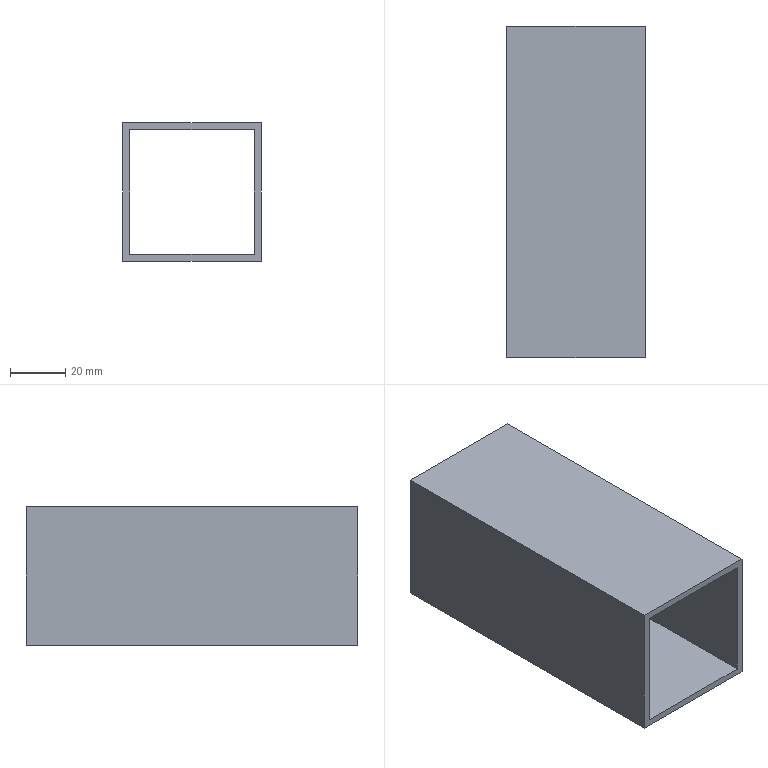Part | STEP file | MB-P-20 | 1 solid | 10 faces | box 50 x 120 x 50 mm | volume 57000 mm3 | plane 10
STEP:
#1=CARTESIAN_POINT('',(2.5,120.,4.5));
#2=VERTEX_POINT('',#1);
#3=CARTESIAN_POINT('',(47.5,120.,4.5));
#4=VERTEX_POINT('',#3);
#5=CARTESIAN_POINT('',(2.5,120.,4.5));
#6=DIRECTION('',(1.,0.,0.));
#7=VECTOR('',#6,1000.);
#8=LINE('',#5,#7);
#9=EDGE_CURVE('',#2,#4,#8,.T.);
#10=ORIENTED_EDGE('',*,*,#9,.T.);
#11=CARTESIAN_POINT('',(47.5,120.,49.5));
#12=VERTEX_POINT('',#11);
#13=CARTESIAN_POINT('',(47.5,120.,4.5));
#14=DIRECTION('',(0.,0.,1.));
#15=VECTOR('',#14,1000.);
#16=LINE('',#13,#15);
#17=EDGE_CURVE('',#4,#12,#16,.T.);
#18=ORIENTED_EDGE('',*,*,#17,.T.);
#19=CARTESIAN_POINT('',(2.5,120.,49.5));
#20=VERTEX_POINT('',#19);
#21=CARTESIAN_POINT('',(47.5,120.,49.5));
#22=DIRECTION('',(-1.,0.,0.));
#23=VECTOR('',#22,1000.);
#24=LINE('',#21,#23);
#25=EDGE_CURVE('',#12,#20,#24,.T.);
#26=ORIENTED_EDGE('',*,*,#25,.T.);
#27=CARTESIAN_POINT('',(2.5,120.,49.5));
#28=DIRECTION('',(0.,0.,-1.));
#29=VECTOR('',#28,1000.);
#30=LINE('',#27,#29);
#31=EDGE_CURVE('',#20,#2,#30,.T.);
#32=ORIENTED_EDGE('',*,*,#31,.T.);
#33=EDGE_LOOP('',(#10,#18,#26,#32));
#34=FACE_BOUND('',#33,.T.);
#35=CARTESIAN_POINT('',(0.,120.,2.));
#36=VERTEX_POINT('',#35);
#37=CARTESIAN_POINT('',(0.,120.,52.));
#38=VERTEX_POINT('',#37);
#39=CARTESIAN_POINT('',(0.,120.,52.));
#40=DIRECTION('',(0.,0.,1.));
#41=VECTOR('',#40,1000.);
#42=LINE('',#39,#41);
#43=EDGE_CURVE('',#36,#38,#42,.T.);
#44=ORIENTED_EDGE('',*,*,#43,.T.);
#45=CARTESIAN_POINT('',(50.,120.,52.));
#46=VERTEX_POINT('',#45);
#47=CARTESIAN_POINT('',(50.,120.,52.));
#48=DIRECTION('',(1.,0.,0.));
#49=VECTOR('',#48,1000.);
#50=LINE('',#47,#49);
#51=EDGE_CURVE('',#38,#46,#50,.T.);
#52=ORIENTED_EDGE('',*,*,#51,.T.);
#53=CARTESIAN_POINT('',(50.,120.,2.));
#54=VERTEX_POINT('',#53);
#55=CARTESIAN_POINT('',(50.,120.,2.));
#56=DIRECTION('',(0.,0.,-1.));
#57=VECTOR('',#56,1000.);
#58=LINE('',#55,#57);
#59=EDGE_CURVE('',#46,#54,#58,.T.);
#60=ORIENTED_EDGE('',*,*,#59,.T.);
#61=CARTESIAN_POINT('',(0.,120.,2.));
#62=DIRECTION('',(-1.,0.,0.));
#63=VECTOR('',#62,1000.);
#64=LINE('',#61,#63);
#65=EDGE_CURVE('',#54,#36,#64,.T.);
#66=ORIENTED_EDGE('',*,*,#65,.T.);
#67=EDGE_LOOP('',(#44,#52,#60,#66));
#68=FACE_OUTER_BOUND('',#67,.T.);
#69=CARTESIAN_POINT('',(25.,120.,27.));
#70=DIRECTION('',(0.,1.,0.));
#71=DIRECTION('',(1.,0.,0.));
#72=AXIS2_PLACEMENT_3D('',#69,#70,#71);
#73=PLANE('',#72);
#74=ADVANCED_FACE('',(#34,#68),#73,.T.);
#75=CARTESIAN_POINT('',(47.5,0.,4.5));
#76=VERTEX_POINT('',#75);
#77=CARTESIAN_POINT('',(2.5,0.,4.5));
#78=VERTEX_POINT('',#77);
#79=CARTESIAN_POINT('',(2.5,0.,4.5));
#80=DIRECTION('',(-1.,0.,0.));
#81=VECTOR('',#80,1000.);
#82=LINE('',#79,#81);
#83=EDGE_CURVE('',#76,#78,#82,.T.);
#84=ORIENTED_EDGE('',*,*,#83,.T.);
#85=CARTESIAN_POINT('',(2.5,0.,49.5));
#86=VERTEX_POINT('',#85);
#87=CARTESIAN_POINT('',(2.5,0.,49.5));
#88=DIRECTION('',(0.,0.,1.));
#89=VECTOR('',#88,1000.);
#90=LINE('',#87,#89);
#91=EDGE_CURVE('',#78,#86,#90,.T.);
#92=ORIENTED_EDGE('',*,*,#91,.T.);
#93=CARTESIAN_POINT('',(47.5,0.,49.5));
#94=VERTEX_POINT('',#93);
#95=CARTESIAN_POINT('',(47.5,0.,49.5));
#96=DIRECTION('',(1.,0.,0.));
#97=VECTOR('',#96,1000.);
#98=LINE('',#95,#97);
#99=EDGE_CURVE('',#86,#94,#98,.T.);
#100=ORIENTED_EDGE('',*,*,#99,.T.);
#101=CARTESIAN_POINT('',(47.5,0.,4.5));
#102=DIRECTION('',(0.,0.,-1.));
#103=VECTOR('',#102,1000.);
#104=LINE('',#101,#103);
#105=EDGE_CURVE('',#94,#76,#104,.T.);
#106=ORIENTED_EDGE('',*,*,#105,.T.);
#107=EDGE_LOOP('',(#84,#92,#100,#106));
#108=FACE_BOUND('',#107,.T.);
#109=CARTESIAN_POINT('',(0.,0.,52.));
#110=VERTEX_POINT('',#109);
#111=CARTESIAN_POINT('',(0.,0.,2.));
#112=VERTEX_POINT('',#111);
#113=CARTESIAN_POINT('',(0.,0.,52.));
#114=DIRECTION('',(0.,0.,-1.));
#115=VECTOR('',#114,1000.);
#116=LINE('',#113,#115);
#117=EDGE_CURVE('',#110,#112,#116,.T.);
#118=ORIENTED_EDGE('',*,*,#117,.T.);
#119=CARTESIAN_POINT('',(50.,0.,2.));
#120=VERTEX_POINT('',#119);
#121=CARTESIAN_POINT('',(0.,0.,2.));
#122=DIRECTION('',(1.,0.,0.));
#123=VECTOR('',#122,1000.);
#124=LINE('',#121,#123);
#125=EDGE_CURVE('',#112,#120,#124,.T.);
#126=ORIENTED_EDGE('',*,*,#125,.T.);
#127=CARTESIAN_POINT('',(50.,0.,52.));
#128=VERTEX_POINT('',#127);
#129=CARTESIAN_POINT('',(50.,0.,2.));
#130=DIRECTION('',(0.,0.,1.));
#131=VECTOR('',#130,1000.);
#132=LINE('',#129,#131);
#133=EDGE_CURVE('',#120,#128,#132,.T.);
#134=ORIENTED_EDGE('',*,*,#133,.T.);
#135=CARTESIAN_POINT('',(50.,0.,52.));
#136=DIRECTION('',(-1.,0.,0.));
#137=VECTOR('',#136,1000.);
#138=LINE('',#135,#137);
#139=EDGE_CURVE('',#128,#110,#138,.T.);
#140=ORIENTED_EDGE('',*,*,#139,.T.);
#141=EDGE_LOOP('',(#118,#126,#134,#140));
#142=FACE_OUTER_BOUND('',#141,.T.);
#143=CARTESIAN_POINT('',(25.,0.,27.));
#144=DIRECTION('',(0.,-1.,0.));
#145=DIRECTION('',(0.,0.,-1.));
#146=AXIS2_PLACEMENT_3D('',#143,#144,#145);
#147=PLANE('',#146);
#148=ADVANCED_FACE('',(#108,#142),#147,.T.);
#149=ORIENTED_EDGE('',*,*,#117,.F.);
#150=CARTESIAN_POINT('',(0.,0.,52.));
#151=DIRECTION('',(0.,1.,0.));
#152=VECTOR('',#151,1000.);
#153=LINE('',#150,#152);
#154=EDGE_CURVE('',#110,#38,#153,.T.);
#155=ORIENTED_EDGE('',*,*,#154,.T.);
#156=ORIENTED_EDGE('',*,*,#43,.F.);
#157=CARTESIAN_POINT('',(0.,0.,2.));
#158=DIRECTION('',(0.,1.,0.));
#159=VECTOR('',#158,1000.);
#160=LINE('',#157,#159);
#161=EDGE_CURVE('',#112,#36,#160,.T.);
#162=ORIENTED_EDGE('',*,*,#161,.F.);
#163=EDGE_LOOP('',(#149,#155,#156,#162));
#164=FACE_OUTER_BOUND('',#163,.T.);
#165=CARTESIAN_POINT('',(0.,0.,2.));
#166=DIRECTION('',(-1.,0.,0.));
#167=DIRECTION('',(0.,0.,1.));
#168=AXIS2_PLACEMENT_3D('',#165,#166,#167);
#169=PLANE('',#168);
#170=ADVANCED_FACE('',(#164),#169,.T.);
#171=ORIENTED_EDGE('',*,*,#139,.F.);
#172=CARTESIAN_POINT('',(50.,0.,52.));
#173=DIRECTION('',(0.,1.,0.));
#174=VECTOR('',#173,1000.);
#175=LINE('',#172,#174);
#176=EDGE_CURVE('',#128,#46,#175,.T.);
#177=ORIENTED_EDGE('',*,*,#176,.T.);
#178=ORIENTED_EDGE('',*,*,#51,.F.);
#179=ORIENTED_EDGE('',*,*,#154,.F.);
#180=EDGE_LOOP('',(#171,#177,#178,#179));
#181=FACE_OUTER_BOUND('',#180,.T.);
#182=CARTESIAN_POINT('',(0.,0.,52.));
#183=DIRECTION('',(0.,0.,1.));
#184=DIRECTION('',(1.,0.,0.));
#185=AXIS2_PLACEMENT_3D('',#182,#183,#184);
#186=PLANE('',#185);
#187=ADVANCED_FACE('',(#181),#186,.T.);
#188=ORIENTED_EDGE('',*,*,#133,.F.);
#189=CARTESIAN_POINT('',(50.,0.,2.));
#190=DIRECTION('',(0.,1.,0.));
#191=VECTOR('',#190,1000.);
#192=LINE('',#189,#191);
#193=EDGE_CURVE('',#120,#54,#192,.T.);
#194=ORIENTED_EDGE('',*,*,#193,.T.);
#195=ORIENTED_EDGE('',*,*,#59,.F.);
#196=ORIENTED_EDGE('',*,*,#176,.F.);
#197=EDGE_LOOP('',(#188,#194,#195,#196));
#198=FACE_OUTER_BOUND('',#197,.T.);
#199=CARTESIAN_POINT('',(50.,0.,52.));
#200=DIRECTION('',(1.,0.,0.));
#201=DIRECTION('',(0.,1.,0.));
#202=AXIS2_PLACEMENT_3D('',#199,#200,#201);
#203=PLANE('',#202);
#204=ADVANCED_FACE('',(#198),#203,.T.);
#205=ORIENTED_EDGE('',*,*,#125,.F.);
#206=ORIENTED_EDGE('',*,*,#161,.T.);
#207=ORIENTED_EDGE('',*,*,#65,.F.);
#208=ORIENTED_EDGE('',*,*,#193,.F.);
#209=EDGE_LOOP('',(#205,#206,#207,#208));
#210=FACE_OUTER_BOUND('',#209,.T.);
#211=CARTESIAN_POINT('',(50.,0.,2.));
#212=DIRECTION('',(0.,0.,-1.));
#213=DIRECTION('',(0.,-1.,0.));
#214=AXIS2_PLACEMENT_3D('',#211,#212,#213);
#215=PLANE('',#214);
#216=ADVANCED_FACE('',(#210),#215,.T.);
#217=ORIENTED_EDGE('',*,*,#83,.F.);
#218=CARTESIAN_POINT('',(47.5,0.,4.5));
#219=DIRECTION('',(0.,1.,0.));
#220=VECTOR('',#219,1000.);
#221=LINE('',#218,#220);
#222=EDGE_CURVE('',#76,#4,#221,.T.);
#223=ORIENTED_EDGE('',*,*,#222,.T.);
#224=ORIENTED_EDGE('',*,*,#9,.F.);
#225=CARTESIAN_POINT('',(2.5,0.,4.5));
#226=DIRECTION('',(0.,1.,0.));
#227=VECTOR('',#226,1000.);
#228=LINE('',#225,#227);
#229=EDGE_CURVE('',#78,#2,#228,.T.);
#230=ORIENTED_EDGE('',*,*,#229,.F.);
#231=EDGE_LOOP('',(#217,#223,#224,#230));
#232=FACE_OUTER_BOUND('',#231,.T.);
#233=CARTESIAN_POINT('',(2.5,0.,4.5));
#234=DIRECTION('',(0.,0.,1.));
#235=DIRECTION('',(1.,0.,0.));
#236=AXIS2_PLACEMENT_3D('',#233,#234,#235);
#237=PLANE('',#236);
#238=ADVANCED_FACE('',(#232),#237,.T.);
#239=ORIENTED_EDGE('',*,*,#105,.F.);
#240=CARTESIAN_POINT('',(47.5,0.,49.5));
#241=DIRECTION('',(0.,1.,0.));
#242=VECTOR('',#241,1000.);
#243=LINE('',#240,#242);
#244=EDGE_CURVE('',#94,#12,#243,.T.);
#245=ORIENTED_EDGE('',*,*,#244,.T.);
#246=ORIENTED_EDGE('',*,*,#17,.F.);
#247=ORIENTED_EDGE('',*,*,#222,.F.);
#248=EDGE_LOOP('',(#239,#245,#246,#247));
#249=FACE_OUTER_BOUND('',#248,.T.);
#250=CARTESIAN_POINT('',(47.5,0.,4.5));
#251=DIRECTION('',(-1.,0.,0.));
#252=DIRECTION('',(0.,0.,1.));
#253=AXIS2_PLACEMENT_3D('',#250,#251,#252);
#254=PLANE('',#253);
#255=ADVANCED_FACE('',(#249),#254,.T.);
#256=ORIENTED_EDGE('',*,*,#99,.F.);
#257=CARTESIAN_POINT('',(2.5,0.,49.5));
#258=DIRECTION('',(0.,1.,0.));
#259=VECTOR('',#258,1000.);
#260=LINE('',#257,#259);
#261=EDGE_CURVE('',#86,#20,#260,.T.);
#262=ORIENTED_EDGE('',*,*,#261,.T.);
#263=ORIENTED_EDGE('',*,*,#25,.F.);
#264=ORIENTED_EDGE('',*,*,#244,.F.);
#265=EDGE_LOOP('',(#256,#262,#263,#264));
#266=FACE_OUTER_BOUND('',#265,.T.);
#267=CARTESIAN_POINT('',(47.5,0.,49.5));
#268=DIRECTION('',(0.,0.,-1.));
#269=DIRECTION('',(0.,-1.,0.));
#270=AXIS2_PLACEMENT_3D('',#267,#268,#269);
#271=PLANE('',#270);
#272=ADVANCED_FACE('',(#266),#271,.T.);
#273=ORIENTED_EDGE('',*,*,#91,.F.);
#274=ORIENTED_EDGE('',*,*,#229,.T.);
#275=ORIENTED_EDGE('',*,*,#31,.F.);
#276=ORIENTED_EDGE('',*,*,#261,.F.);
#277=EDGE_LOOP('',(#273,#274,#275,#276));
#278=FACE_OUTER_BOUND('',#277,.T.);
#279=CARTESIAN_POINT('',(2.5,0.,49.5));
#280=DIRECTION('',(1.,0.,0.));
#281=DIRECTION('',(0.,0.,1.));
#282=AXIS2_PLACEMENT_3D('',#279,#280,#281);
#283=PLANE('',#282);
#284=ADVANCED_FACE('',(#278),#283,.T.);
#285=CLOSED_SHELL('',(#74,#148,#170,#187,#204,#216,#238,#255,#272,#284));
#286=MANIFOLD_SOLID_BREP('',#285);
#287=CARTESIAN_POINT('',(0.,0.,0.));
#288=DIRECTION('',(0.,0.,1.));
#289=DIRECTION('',(1.,0.,0.));
#290=AXIS2_PLACEMENT_3D('',#287,#288,#289);
#291=(LENGTH_UNIT()NAMED_UNIT(*)SI_UNIT(.MILLI.,.METRE.));
#292=UNCERTAINTY_MEASURE_WITH_UNIT(LENGTH_MEASURE(0.00001),#291,'','');
#293=(NAMED_UNIT(*)PLANE_ANGLE_UNIT()SI_UNIT($,.RADIAN.));
#294=(NAMED_UNIT(*)SI_UNIT($,.STERADIAN.)SOLID_ANGLE_UNIT());
#295=(GEOMETRIC_REPRESENTATION_CONTEXT(3)GLOBAL_UNCERTAINTY_ASSIGNED_CONTEXT((#292))GLOBAL_UNIT_ASSIGNED_CONTEXT((#291,#293,#294))REPRESENTATION_CONTEXT('',''));
#296=ADVANCED_BREP_SHAPE_REPRESENTATION('',(#286,#290),#295);